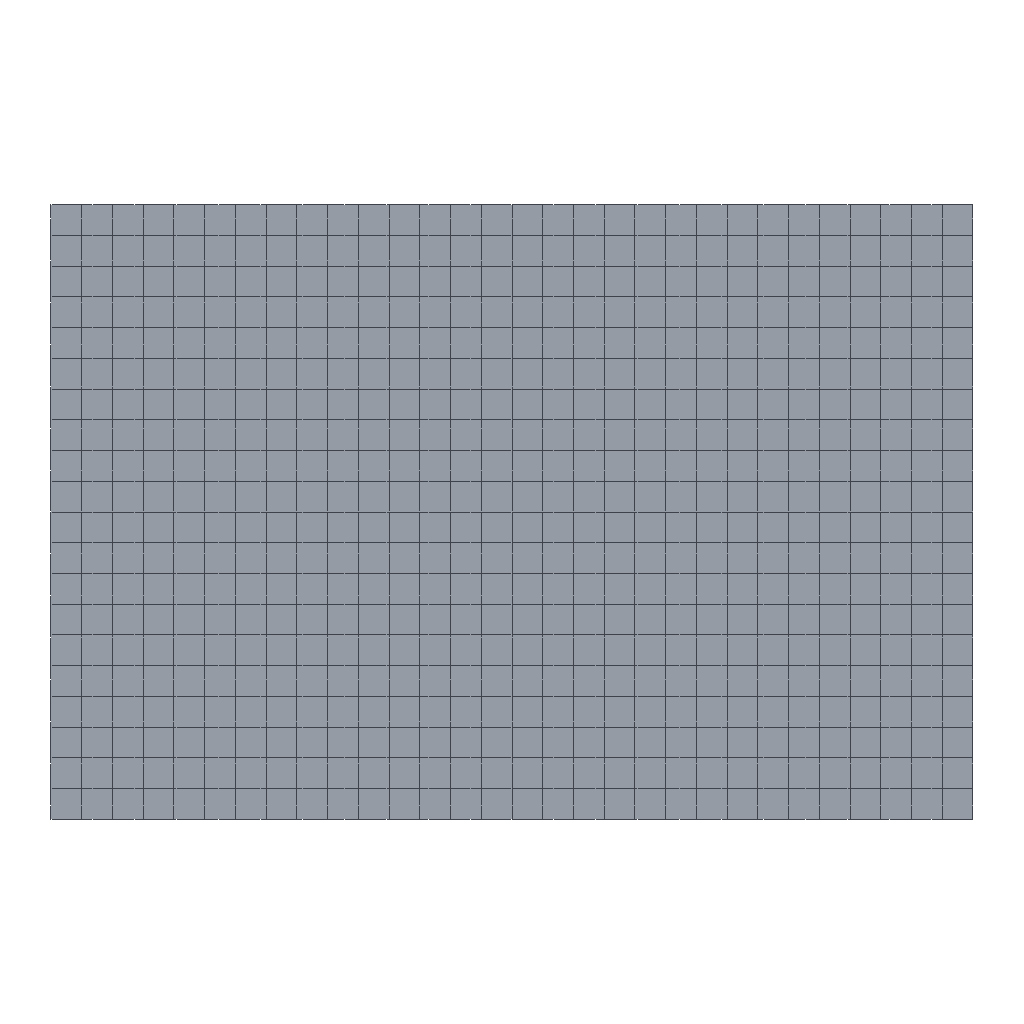Simulation study | abaqus
Set-up summary:
category,name,step,type,value,unit,region
solver,abaqus,,Abaqus/CAE 2024
units,mm-N-s-tonne (MPa),,inferred,E=210000 density=
analysis,InContact,,static,nlgeom=True; time_period=1
analysis,Apply Load,,static,nlgeom=True; time_period=1
mesh,nodes,,,652
mesh,elements,,,600
element_type,CPS4I,,,600
material,Material-1,,E,210000
material,Material-1,,nu,0.3
section,Material-1,,solid section,,,_PickedSet2
load,Load-1,InContact,concentrated force,"10 [dir=(0, -1, 0)]",,Set-Cylinder_Ref
load,Load-1,Apply Load,concentrated force,"6000 [dir=(0, -1, 0)]",,Set-Cylinder_Ref
bc,BC-Cylinder,initial,fixed,"[dofs=rz,x n=2]",,Set-Cylinder_Ref
bc,BC-X-Fix,initial,fixed,[dofs=x],,Set-X-Fix
bc,BC-XY-Fix,initial,fixed,"[dofs=x,y n=2]",,Set-XY_Fix
contact,Int-1,initial,contact pair surface to surface,interaction=IntProp-NoFriciton,,Surf-Plane / Cylinder-1.Surf-Cylinder
constraint,rigid body,,,1
Abaqus input file, long lists of numbers shortened:
*Heading
** Job name: deck Model name: Model-1
** Generated by: Abaqus/CAE 2024
*Preprint, echo=NO, model=NO, history=NO, contact=NO
**
** PARTS
**
*Part, name=Cylinder
*End Part
**
*Part, name=Plane
*Node
      1,          45.,           0.
      2,         43.5,           0.
** (649 more lines like these left out)
*Element, type=CPS4I
  1,   1,   2,  33,  32
  2,   2,   3,  34,  33
** (598 more lines like these left out)
*Nset, nset=_PickedSet2, internal, generate
   1,  651,    1
*Elset, elset=_PickedSet2, internal, generate
   1,  600,    1
** Section: Section-1
*Solid Section, elset=_PickedSet2, material=Material-1
,
*End Part
**
**
** ASSEMBLY
**
*Assembly, name=Assembly
**
*Instance, name=Cylinder-1, part=Cylinder
*Node
      1, -1.83690953e-15,           0.,           0.
*Nset, nset=Cylinder-1-RefPt_, internal
1,
*Surface, type=SEGMENTS, name=Surf-Cylinder
START,          10.,          10.
 CIRCL,           0.,           0.,           0.,          10.
*Rigid Body, ref node=Cylinder-1-RefPt_, analytical surface=Surf-Cylinder
*End Instance
**
*Instance, name=Plane-1, part=Plane
*End Instance
**
*Nset, nset=Set-Cylinder_Ref, instance=Cylinder-1
 1,
*Nset, nset=Set-X-Fix, instance=Plane-1, generate
  31,  651,   31
*Elset, elset=Set-X-Fix, instance=Plane-1, generate
  30,  600,   30
*Nset, nset=Set-XY_Fix, instance=Plane-1, generate
 621,  651,    1
*Elset, elset=Set-XY_Fix, instance=Plane-1, generate
 571,  600,    1
*Elset, elset=_Surf-Plane_S1, internal, instance=Plane-1, generate
  1,  30,   1
*Surface, type=ELEMENT, name=Surf-Plane
_Surf-Plane_S1, S1
*End Assembly
**
** MATERIALS
**
*Material, name=Material-1
*Elastic
210000., 0.3
**
** INTERACTION PROPERTIES
**
*Surface Interaction, name=IntProp-NoFriciton
1.,
**
** BOUNDARY CONDITIONS
**
** Name: BC-Cylinder Type: Displacement/Rotation
*Boundary
Set-Cylinder_Ref, 1, 1
Set-Cylinder_Ref, 6, 6
** Name: BC-X-Fix Type: Displacement/Rotation
*Boundary
Set-X-Fix, 1, 1
** Name: BC-XY-Fix Type: Displacement/Rotation
*Boundary
Set-XY_Fix, 1, 1
Set-XY_Fix, 2, 2
**
** INTERACTIONS
**
** Interaction: Int-1
*Contact Pair, interaction=IntProp-NoFriciton, type=SURFACE TO SURFACE
Surf-Plane, Cylinder-1.Surf-Cylinder
** ----------------------------------------------------------------
**
** STEP: InContact
**
*Step, name=InContact, nlgeom=YES
*Static
1., 1., 1e-05, 1.
**
** LOADS
**
** Name: Load-1   Type: Concentrated force
*Cload
Set-Cylinder_Ref, 2, -10.
**
** OUTPUT REQUESTS
**
*Restart, write, frequency=0
*Print, solve=NO
**
** FIELD OUTPUT: F-Output-1
**
*Output, field, variable=PRESELECT
**
** HISTORY OUTPUT: H-Output-1
**
*Output, history, variable=PRESELECT
*End Step
** ----------------------------------------------------------------
**
** STEP: Apply Load
**
*Step, name="Apply Load", nlgeom=YES
*Static
1., 1., 1e-05, 1.
**
** LOADS
**
** Name: Load-1   Type: Concentrated force
*Cload
Set-Cylinder_Ref, 2, -6000.
**
** OUTPUT REQUESTS
**
*Restart, write, frequency=0
**
** FIELD OUTPUT: F-Output-1
**
*Output, field, variable=PRESELECT
**
** HISTORY OUTPUT: H-Output-1
**
*Output, history, variable=PRESELECT
*End Step
Results summary:
result,odb.job_status,,,JOB_STATUS_COMPLETED_SUCCESSFULLY,"consistent, unstated (Abaqus has no unit system)"
result,steps[0].procedure,InContact,,*STATIC,"consistent, unstated (Abaqus has no unit system)"
result,steps[0].time_period,InContact,,1,"consistent, unstated (Abaqus has no unit system)"
result,steps[0].n_frames,InContact,,8,"consistent, unstated (Abaqus has no unit system)"
result,steps[0].last_frame.id,InContact,,7,"consistent, unstated (Abaqus has no unit system)"
result,steps[0].last_frame.value,InContact,,1,"consistent, unstated (Abaqus has no unit system)"
result,steps[0].last_frame.description,InContact,,Increment      7: Step Time =    1.000,"consistent, unstated (Abaqus has no unit system)"
result,steps[0].completed,InContact,,True,"consistent, unstated (Abaqus has no unit system)"
result,steps[0].max_U_magnitude,InContact,,0.009629,"consistent, unstated (Abaqus has no unit system)"
result,steps[0].max_S_mises,InContact,,9.096,"consistent, unstated (Abaqus has no unit system)"
result,steps[0].RF_sum[1],InContact,,4.91738e-07,"consistent, unstated (Abaqus has no unit system)"
result,steps[0].RF_sum[2],InContact,,10,"consistent, unstated (Abaqus has no unit system)"
result,steps[0].diagnostic.n_increments,InContact,,7,"consistent, unstated (Abaqus has no unit system)"
result,steps[1].procedure,Apply Load,,*STATIC,"consistent, unstated (Abaqus has no unit system)"
result,steps[1].time_period,Apply Load,,1,"consistent, unstated (Abaqus has no unit system)"
result,steps[1].n_frames,Apply Load,,2,"consistent, unstated (Abaqus has no unit system)"
result,steps[1].last_frame.id,Apply Load,,1,"consistent, unstated (Abaqus has no unit system)"
result,steps[1].last_frame.value,Apply Load,,1,"consistent, unstated (Abaqus has no unit system)"
result,steps[1].last_frame.description,Apply Load,,Increment      1: Step Time =    1.000,"consistent, unstated (Abaqus has no unit system)"
result,steps[1].completed,Apply Load,,True,"consistent, unstated (Abaqus has no unit system)"
result,steps[1].max_U_magnitude,Apply Load,,0.1565,"consistent, unstated (Abaqus has no unit system)"
result,steps[1].max_S_mises,Apply Load,,5422.04,"consistent, unstated (Abaqus has no unit system)"
result,steps[1].RF_sum[1],Apply Load,,0.01005,"consistent, unstated (Abaqus has no unit system)"
result,steps[1].RF_sum[2],Apply Load,,6000,"consistent, unstated (Abaqus has no unit system)"